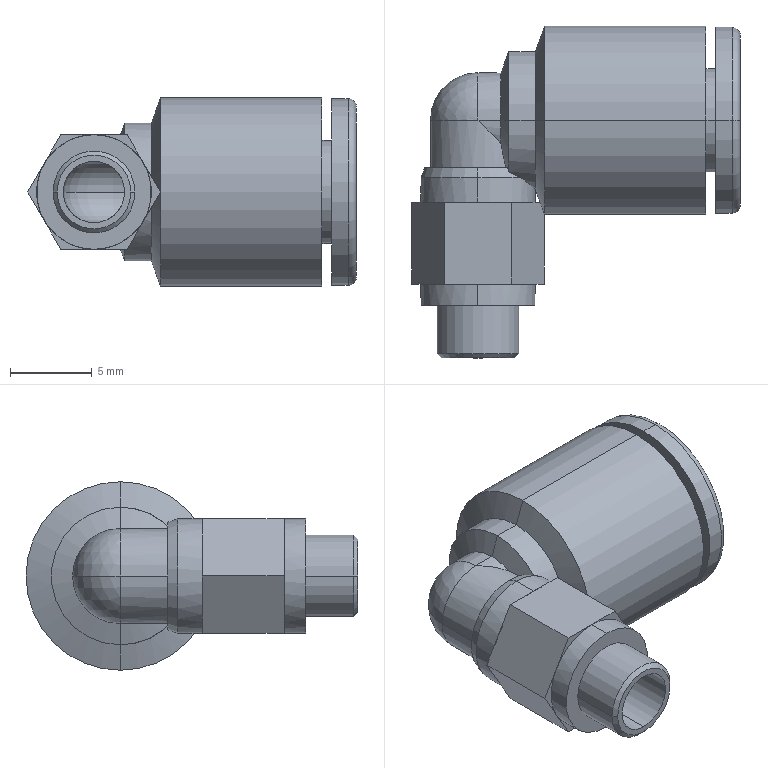Part | SolidWorks | 1 solid | 67 faces | box 20.041 x 20.25 x 11.5 mm | volume 1277 mm3 | plane 25 | cylinder 24 | cone 10 | torus 6 | sphere 2 | commonest cylinder face diameters 5.8 x5 7 x4 8.4 x3 3.75 x2 5 x2 6 x2